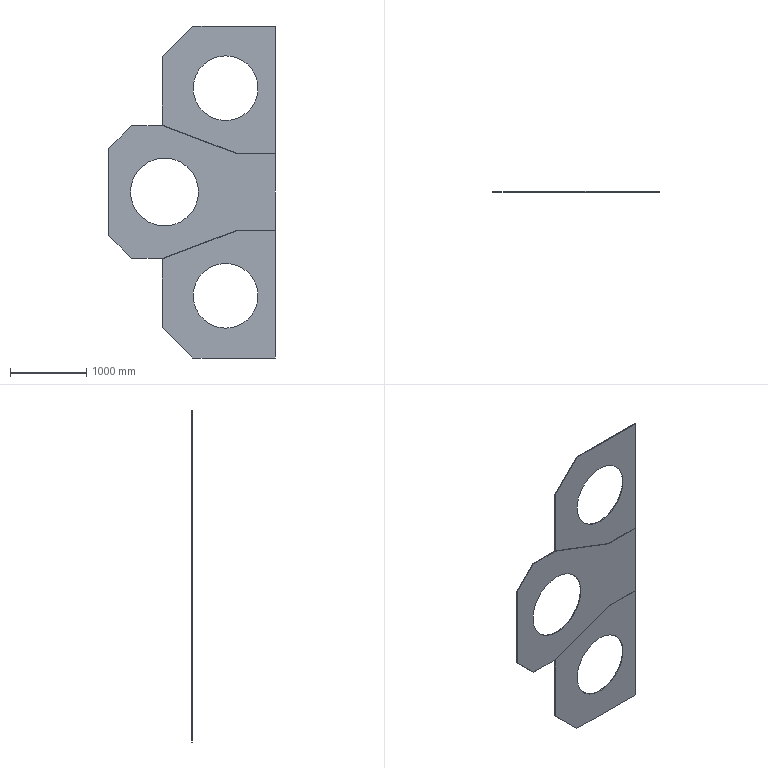Part | STEP file | 计量Pad 1 | 3 solids | 34 faces | box 2185 x 10 x 4350 mm | volume 56422097 mm3 | plane 28 | cylinder 6 | commonest cylinder face diameters 850 x4 890 x2